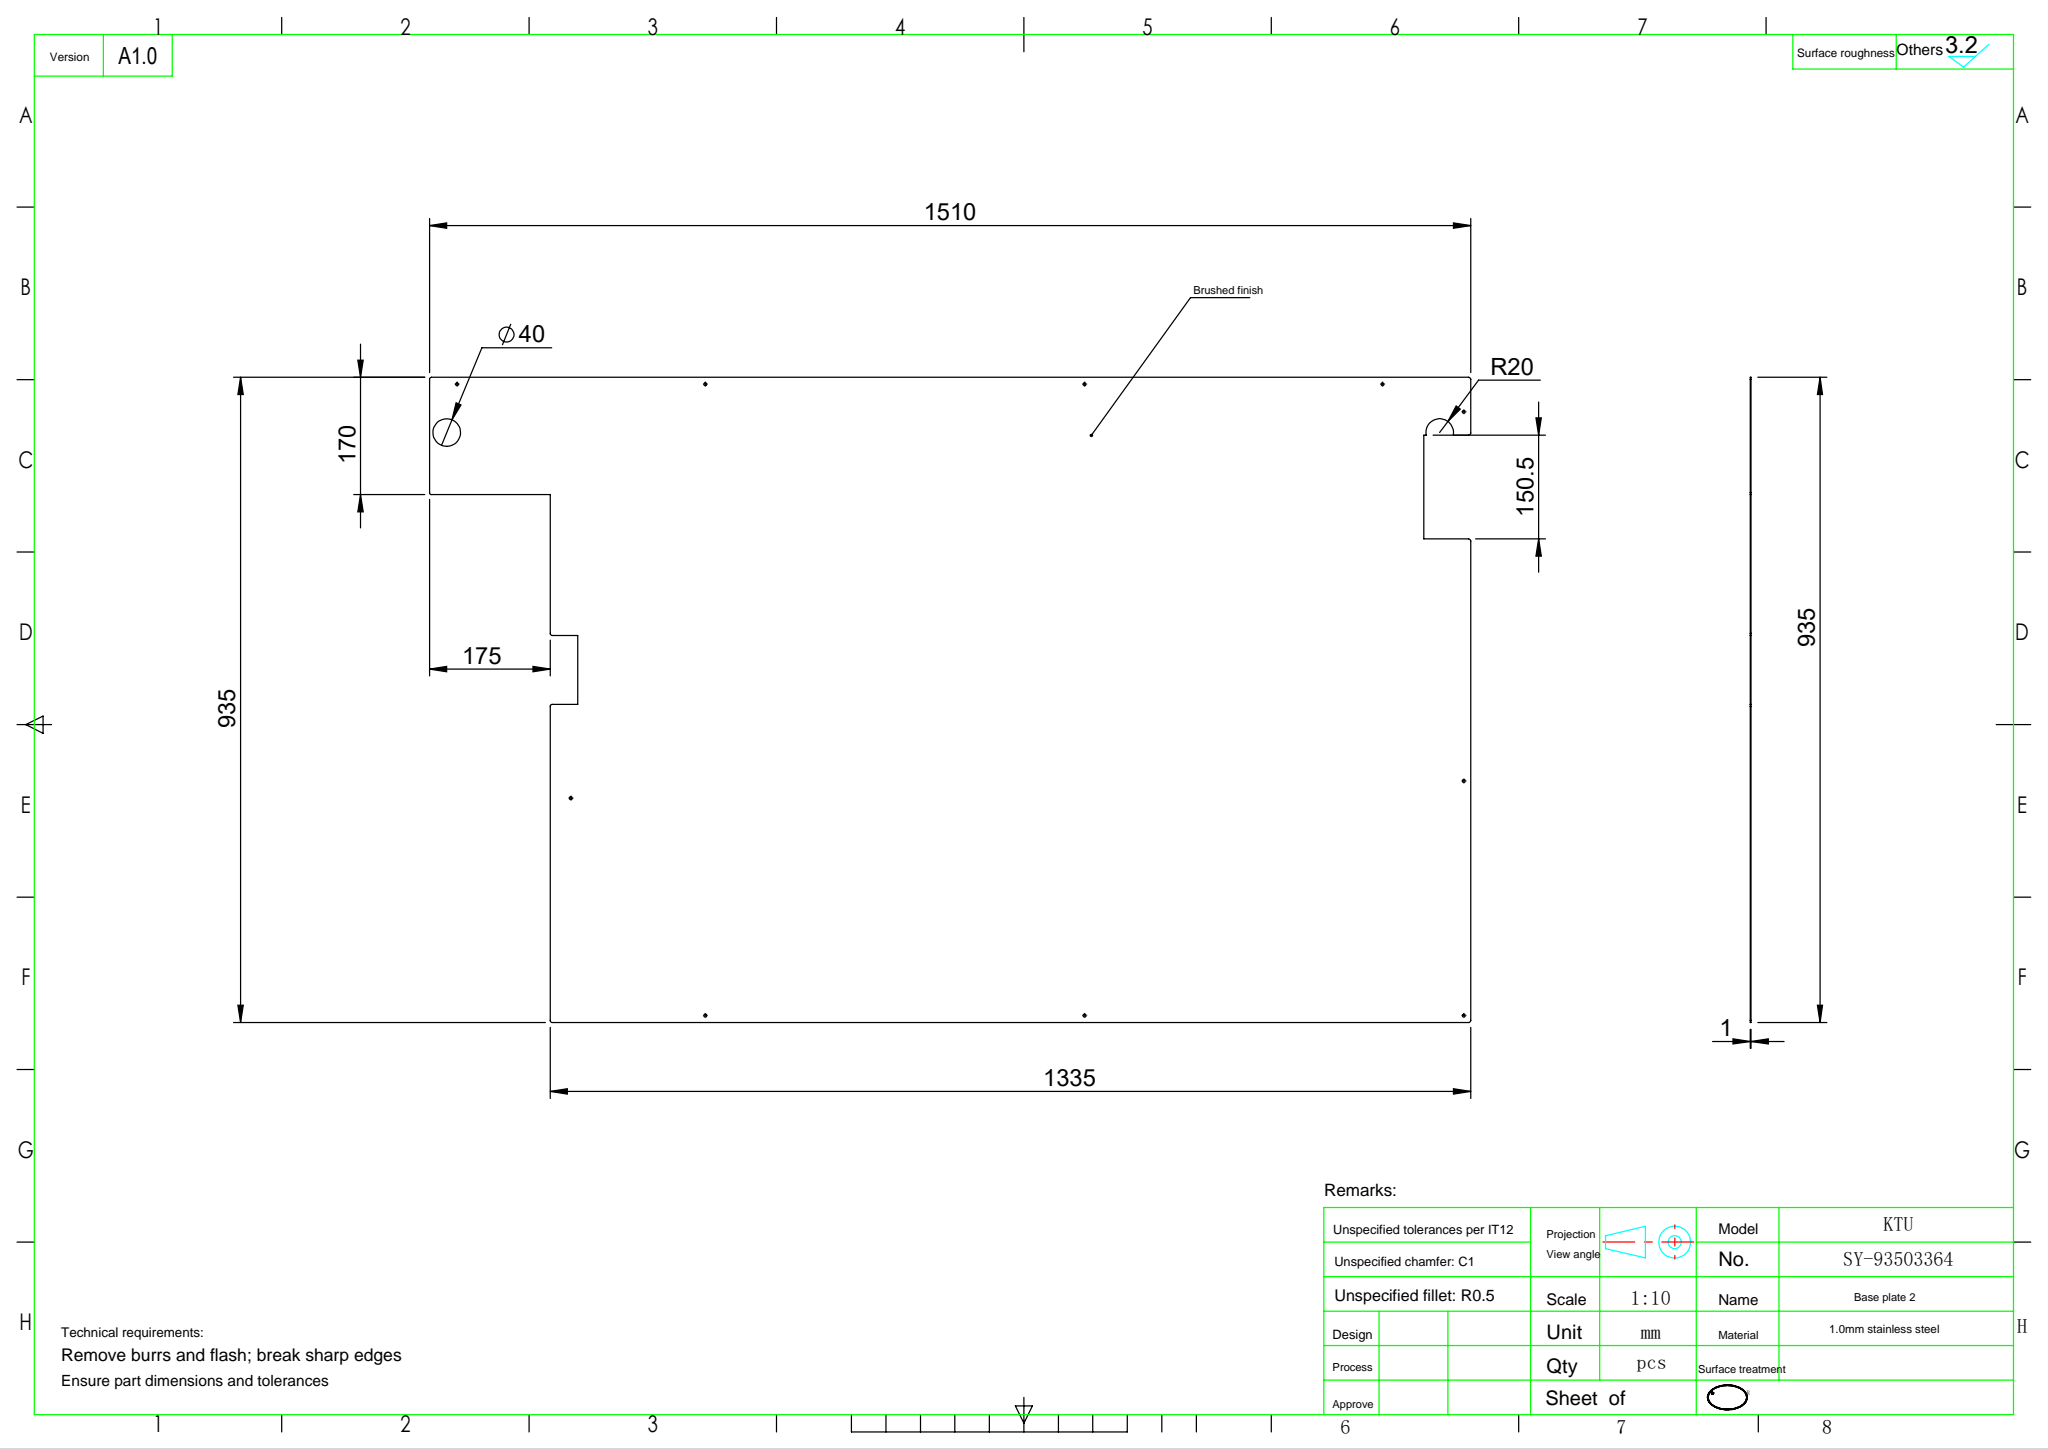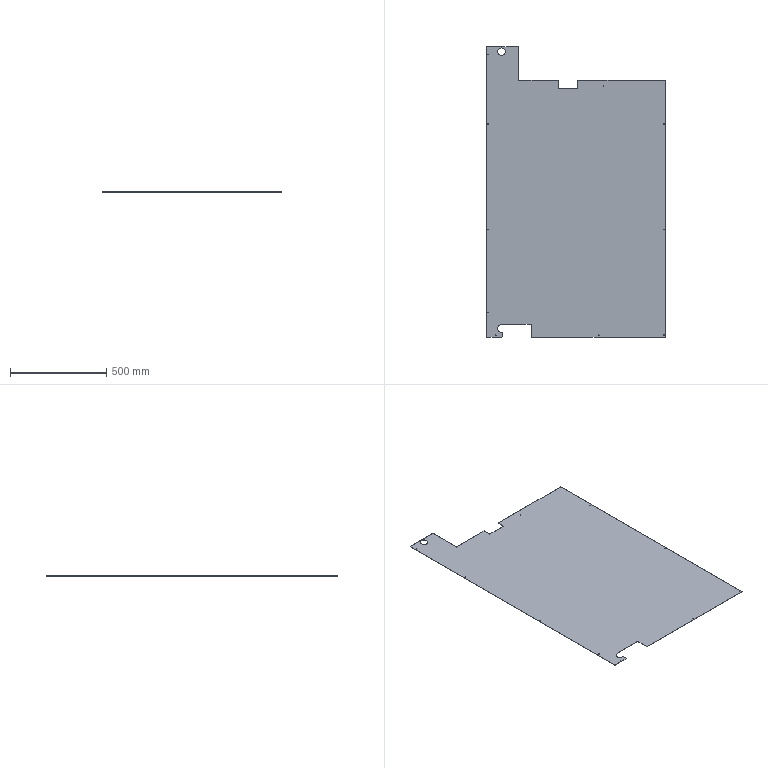Part | SolidWorks | features ICE 4, Cut 2, Fillet 1, FlatPattern 1, SMBaseFlange 1, SheetMetal 1 | 1 solid | 49 faces | box 935 x 1510 x 1 mm | volume 1261551 mm3 | cylinder 32 | plane 17 | commonest cylinder face diameters 4.2 x20 6 x9 40 x3